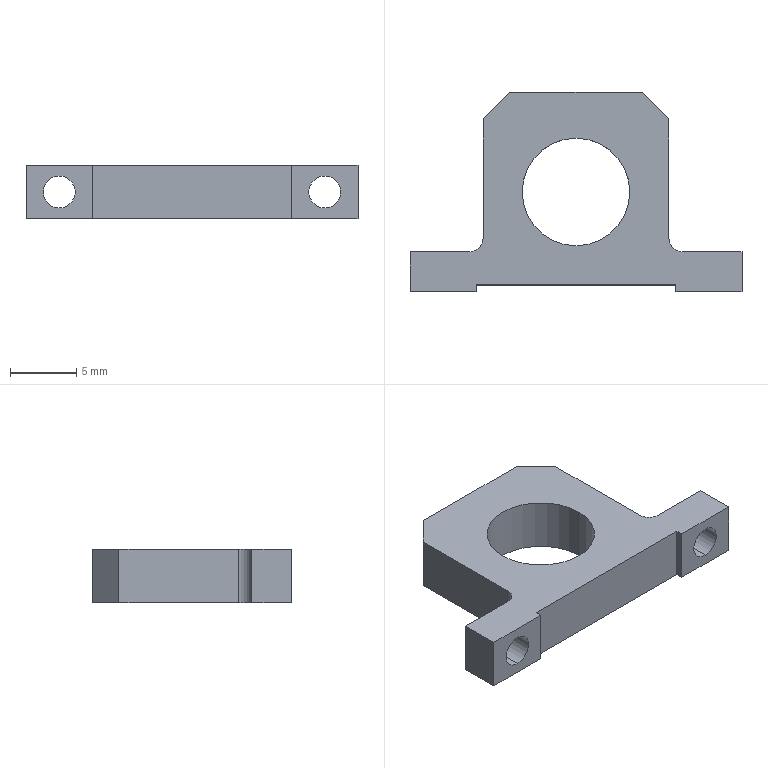Part | SolidWorks | features ICE 3, MoveFace 2, Chamfer 1, Cut 1, Extrusion 1, Fillet 1 | 1 solid | 24 faces | box 25 x 15 x 4 mm | volume 694.454 mm3 | plane 16 | cylinder 8 | commonest cylinder face diameters 2.4 x4 2 x2 8.1 x2
STEP:
#1=CARTESIAN_POINT('',(-10.,-7.5,0.8));
#2=VERTEX_POINT('',#1);
#3=CARTESIAN_POINT('',(-10.,-7.5,3.2));
#4=VERTEX_POINT('',#3);
#5=CARTESIAN_POINT('',(-10.,-7.5,2.));
#6=DIRECTION('',(0.,1.,0.));
#7=DIRECTION('',(0.,0.,1.));
#8=AXIS2_PLACEMENT_3D('',#5,#6,#7);
#9=CIRCLE('',#8,1.2);
#10=EDGE_CURVE('',#2,#4,#9,.T.);
#11=ORIENTED_EDGE('',*,*,#10,.F.);
#12=CARTESIAN_POINT('',(-10.,-4.5,0.8));
#13=VERTEX_POINT('',#12);
#14=CARTESIAN_POINT('',(-10.,-14.5,0.8));
#15=DIRECTION('',(0.,1.,0.));
#16=VECTOR('',#15,1000.);
#17=LINE('',#14,#16);
#18=EDGE_CURVE('',#2,#13,#17,.T.);
#19=ORIENTED_EDGE('',*,*,#18,.T.);
#20=CARTESIAN_POINT('',(-10.,-4.5,3.2));
#21=VERTEX_POINT('',#20);
#22=CARTESIAN_POINT('',(-10.,-4.5,2.));
#23=DIRECTION('',(0.,1.,0.));
#24=DIRECTION('',(0.,0.,1.));
#25=AXIS2_PLACEMENT_3D('',#22,#23,#24);
#26=CIRCLE('',#25,1.2);
#27=EDGE_CURVE('',#13,#21,#26,.T.);
#28=ORIENTED_EDGE('',*,*,#27,.T.);
#29=CARTESIAN_POINT('',(-10.,-14.5,3.2));
#30=DIRECTION('',(0.,1.,0.));
#31=VECTOR('',#30,1000.);
#32=LINE('',#29,#31);
#33=EDGE_CURVE('',#4,#21,#32,.T.);
#34=ORIENTED_EDGE('',*,*,#33,.F.);
#35=EDGE_LOOP('',(#11,#19,#28,#34));
#36=FACE_OUTER_BOUND('',#35,.T.);
#37=CARTESIAN_POINT('',(-10.,-14.5,2.));
#38=DIRECTION('',(0.,1.,0.));
#39=DIRECTION('',(0.,0.,1.));
#40=AXIS2_PLACEMENT_3D('',#37,#38,#39);
#41=CYLINDRICAL_SURFACE('',#40,1.2);
#42=ADVANCED_FACE('',(#36),#41,.F.);
#43=CARTESIAN_POINT('',(10.,-7.5,0.8));
#44=VERTEX_POINT('',#43);
#45=CARTESIAN_POINT('',(10.,-7.5,3.2));
#46=VERTEX_POINT('',#45);
#47=CARTESIAN_POINT('',(10.,-7.5,2.));
#48=DIRECTION('',(0.,1.,0.));
#49=DIRECTION('',(0.,0.,1.));
#50=AXIS2_PLACEMENT_3D('',#47,#48,#49);
#51=CIRCLE('',#50,1.2);
#52=EDGE_CURVE('',#44,#46,#51,.T.);
#53=ORIENTED_EDGE('',*,*,#52,.F.);
#54=CARTESIAN_POINT('',(10.,-4.5,0.8));
#55=VERTEX_POINT('',#54);
#56=CARTESIAN_POINT('',(10.,-14.5,0.8));
#57=DIRECTION('',(0.,1.,0.));
#58=VECTOR('',#57,1000.);
#59=LINE('',#56,#58);
#60=EDGE_CURVE('',#44,#55,#59,.T.);
#61=ORIENTED_EDGE('',*,*,#60,.T.);
#62=CARTESIAN_POINT('',(10.,-4.5,3.2));
#63=VERTEX_POINT('',#62);
#64=CARTESIAN_POINT('',(10.,-4.5,2.));
#65=DIRECTION('',(0.,1.,0.));
#66=DIRECTION('',(0.,0.,1.));
#67=AXIS2_PLACEMENT_3D('',#64,#65,#66);
#68=CIRCLE('',#67,1.2);
#69=EDGE_CURVE('',#55,#63,#68,.T.);
#70=ORIENTED_EDGE('',*,*,#69,.T.);
#71=CARTESIAN_POINT('',(10.,-14.5,3.2));
#72=DIRECTION('',(0.,1.,0.));
#73=VECTOR('',#72,1000.);
#74=LINE('',#71,#73);
#75=EDGE_CURVE('',#46,#63,#74,.T.);
#76=ORIENTED_EDGE('',*,*,#75,.F.);
#77=EDGE_LOOP('',(#53,#61,#70,#76));
#78=FACE_OUTER_BOUND('',#77,.T.);
#79=CARTESIAN_POINT('',(10.,-14.5,2.));
#80=DIRECTION('',(0.,1.,0.));
#81=DIRECTION('',(0.,0.,1.));
#82=AXIS2_PLACEMENT_3D('',#79,#80,#81);
#83=CYLINDRICAL_SURFACE('',#82,1.2);
#84=ADVANCED_FACE('',(#78),#83,.F.);
#85=CARTESIAN_POINT('',(-4.05,0.,0.));
#86=VERTEX_POINT('',#85);
#87=CARTESIAN_POINT('',(4.05,0.,0.));
#88=VERTEX_POINT('',#87);
#89=CARTESIAN_POINT('',(0.,0.,0.));
#90=DIRECTION('',(0.,0.,1.));
#91=DIRECTION('',(1.,0.,0.));
#92=AXIS2_PLACEMENT_3D('',#89,#90,#91);
#93=CIRCLE('',#92,4.05);
#94=EDGE_CURVE('',#86,#88,#93,.T.);
#95=ORIENTED_EDGE('',*,*,#94,.F.);
#96=CARTESIAN_POINT('',(-4.05,0.,4.));
#97=VERTEX_POINT('',#96);
#98=CARTESIAN_POINT('',(-4.05,0.,0.));
#99=DIRECTION('',(0.,0.,1.));
#100=VECTOR('',#99,1000.);
#101=LINE('',#98,#100);
#102=EDGE_CURVE('',#86,#97,#101,.T.);
#103=ORIENTED_EDGE('',*,*,#102,.T.);
#104=CARTESIAN_POINT('',(4.05,0.,4.));
#105=VERTEX_POINT('',#104);
#106=CARTESIAN_POINT('',(0.,0.,4.));
#107=DIRECTION('',(0.,0.,1.));
#108=DIRECTION('',(1.,0.,0.));
#109=AXIS2_PLACEMENT_3D('',#106,#107,#108);
#110=CIRCLE('',#109,4.05);
#111=EDGE_CURVE('',#97,#105,#110,.T.);
#112=ORIENTED_EDGE('',*,*,#111,.T.);
#113=CARTESIAN_POINT('',(4.05,0.,0.));
#114=DIRECTION('',(0.,0.,1.));
#115=VECTOR('',#114,1000.);
#116=LINE('',#113,#115);
#117=EDGE_CURVE('',#88,#105,#116,.T.);
#118=ORIENTED_EDGE('',*,*,#117,.F.);
#119=EDGE_LOOP('',(#95,#103,#112,#118));
#120=FACE_OUTER_BOUND('',#119,.T.);
#121=CARTESIAN_POINT('',(0.,0.,0.));
#122=DIRECTION('',(0.,0.,1.));
#123=DIRECTION('',(1.,0.,0.));
#124=AXIS2_PLACEMENT_3D('',#121,#122,#123);
#125=CYLINDRICAL_SURFACE('',#124,4.05);
#126=ADVANCED_FACE('',(#120),#125,.F.);
#127=CARTESIAN_POINT('',(-10.,-7.5,2.));
#128=DIRECTION('',(0.,1.,0.));
#129=DIRECTION('',(0.,0.,1.));
#130=AXIS2_PLACEMENT_3D('',#127,#128,#129);
#131=CIRCLE('',#130,1.2);
#132=EDGE_CURVE('',#4,#2,#131,.T.);
#133=ORIENTED_EDGE('',*,*,#132,.T.);
#134=ORIENTED_EDGE('',*,*,#10,.T.);
#135=EDGE_LOOP('',(#133,#134));
#136=FACE_BOUND('',#135,.T.);
#137=CARTESIAN_POINT('',(-12.5,-7.5,0.));
#138=VERTEX_POINT('',#137);
#139=CARTESIAN_POINT('',(-7.5,-7.5,0.));
#140=VERTEX_POINT('',#139);
#141=CARTESIAN_POINT('',(-7.5,-7.5,0.));
#142=DIRECTION('',(1.,0.,0.));
#143=VECTOR('',#142,1000.);
#144=LINE('',#141,#143);
#145=EDGE_CURVE('',#138,#140,#144,.T.);
#146=ORIENTED_EDGE('',*,*,#145,.T.);
#147=CARTESIAN_POINT('',(-7.5,-7.5,4.));
#148=VERTEX_POINT('',#147);
#149=CARTESIAN_POINT('',(-7.5,-7.5,-6.));
#150=DIRECTION('',(0.,0.,1.));
#151=VECTOR('',#150,1000.);
#152=LINE('',#149,#151);
#153=EDGE_CURVE('',#140,#148,#152,.T.);
#154=ORIENTED_EDGE('',*,*,#153,.T.);
#155=CARTESIAN_POINT('',(-12.5,-7.5,4.));
#156=VERTEX_POINT('',#155);
#157=CARTESIAN_POINT('',(-7.5,-7.5,4.));
#158=DIRECTION('',(1.,0.,0.));
#159=VECTOR('',#158,1000.);
#160=LINE('',#157,#159);
#161=EDGE_CURVE('',#156,#148,#160,.T.);
#162=ORIENTED_EDGE('',*,*,#161,.F.);
#163=CARTESIAN_POINT('',(-12.5,-7.5,0.));
#164=DIRECTION('',(0.,0.,-1.));
#165=VECTOR('',#164,1000.);
#166=LINE('',#163,#165);
#167=EDGE_CURVE('',#156,#138,#166,.T.);
#168=ORIENTED_EDGE('',*,*,#167,.T.);
#169=EDGE_LOOP('',(#146,#154,#162,#168));
#170=FACE_OUTER_BOUND('',#169,.T.);
#171=CARTESIAN_POINT('',(-7.5,-7.5,4.));
#172=DIRECTION('',(0.,1.,0.));
#173=DIRECTION('',(0.,0.,1.));
#174=AXIS2_PLACEMENT_3D('',#171,#172,#173);
#175=PLANE('',#174);
#176=ADVANCED_FACE('',(#136,#170),#175,.F.);
#177=CARTESIAN_POINT('',(7.,-3.5,4.));
#178=VERTEX_POINT('',#177);
#179=CARTESIAN_POINT('',(7.,5.5,4.));
#180=VERTEX_POINT('',#179);
#181=CARTESIAN_POINT('',(7.,7.5,4.));
#182=DIRECTION('',(0.,1.,0.));
#183=VECTOR('',#182,1000.);
#184=LINE('',#181,#183);
#185=EDGE_CURVE('',#178,#180,#184,.T.);
#186=ORIENTED_EDGE('',*,*,#185,.F.);
#187=CARTESIAN_POINT('',(7.,-3.5,0.));
#188=VERTEX_POINT('',#187);
#189=CARTESIAN_POINT('',(7.,-3.5,4.));
#190=DIRECTION('',(0.,0.,-1.));
#191=VECTOR('',#190,1000.);
#192=LINE('',#189,#191);
#193=EDGE_CURVE('',#178,#188,#192,.T.);
#194=ORIENTED_EDGE('',*,*,#193,.T.);
#195=CARTESIAN_POINT('',(7.,5.5,0.));
#196=VERTEX_POINT('',#195);
#197=CARTESIAN_POINT('',(7.,7.5,0.));
#198=DIRECTION('',(0.,1.,0.));
#199=VECTOR('',#198,1000.);
#200=LINE('',#197,#199);
#201=EDGE_CURVE('',#188,#196,#200,.T.);
#202=ORIENTED_EDGE('',*,*,#201,.T.);
#203=CARTESIAN_POINT('',(7.,5.5,4.));
#204=DIRECTION('',(0.,0.,1.));
#205=VECTOR('',#204,1000.);
#206=LINE('',#203,#205);
#207=EDGE_CURVE('',#196,#180,#206,.T.);
#208=ORIENTED_EDGE('',*,*,#207,.T.);
#209=EDGE_LOOP('',(#186,#194,#202,#208));
#210=FACE_OUTER_BOUND('',#209,.T.);
#211=CARTESIAN_POINT('',(7.,7.5,4.));
#212=DIRECTION('',(-1.,0.,0.));
#213=DIRECTION('',(0.,0.,1.));
#214=AXIS2_PLACEMENT_3D('',#211,#212,#213);
#215=PLANE('',#214);
#216=ADVANCED_FACE('',(#210),#215,.F.);
#217=CARTESIAN_POINT('',(5.,7.5,4.));
#218=VERTEX_POINT('',#217);
#219=CARTESIAN_POINT('',(-5.,7.5,4.));
#220=VERTEX_POINT('',#219);
#221=CARTESIAN_POINT('',(-7.5,7.5,4.));
#222=DIRECTION('',(-1.,0.,0.));
#223=VECTOR('',#222,1000.);
#224=LINE('',#221,#223);
#225=EDGE_CURVE('',#218,#220,#224,.T.);
#226=ORIENTED_EDGE('',*,*,#225,.F.);
#227=CARTESIAN_POINT('',(5.,7.5,0.));
#228=VERTEX_POINT('',#227);
#229=CARTESIAN_POINT('',(5.,7.5,4.));
#230=DIRECTION('',(0.,0.,-1.));
#231=VECTOR('',#230,1000.);
#232=LINE('',#229,#231);
#233=EDGE_CURVE('',#218,#228,#232,.T.);
#234=ORIENTED_EDGE('',*,*,#233,.T.);
#235=CARTESIAN_POINT('',(-5.,7.5,0.));
#236=VERTEX_POINT('',#235);
#237=CARTESIAN_POINT('',(-7.5,7.5,0.));
#238=DIRECTION('',(-1.,0.,0.));
#239=VECTOR('',#238,1000.);
#240=LINE('',#237,#239);
#241=EDGE_CURVE('',#228,#236,#240,.T.);
#242=ORIENTED_EDGE('',*,*,#241,.T.);
#243=CARTESIAN_POINT('',(-5.,7.5,4.));
#244=DIRECTION('',(0.,0.,1.));
#245=VECTOR('',#244,1000.);
#246=LINE('',#243,#245);
#247=EDGE_CURVE('',#236,#220,#246,.T.);
#248=ORIENTED_EDGE('',*,*,#247,.T.);
#249=EDGE_LOOP('',(#226,#234,#242,#248));
#250=FACE_OUTER_BOUND('',#249,.T.);
#251=CARTESIAN_POINT('',(-7.5,7.5,4.));
#252=DIRECTION('',(0.,-1.,0.));
#253=DIRECTION('',(0.,0.,-1.));
#254=AXIS2_PLACEMENT_3D('',#251,#252,#253);
#255=PLANE('',#254);
#256=ADVANCED_FACE('',(#250),#255,.F.);
#257=CARTESIAN_POINT('',(-7.,5.5,0.));
#258=VERTEX_POINT('',#257);
#259=CARTESIAN_POINT('',(-7.,-3.5,0.));
#260=VERTEX_POINT('',#259);
#261=CARTESIAN_POINT('',(-7.,7.5,0.));
#262=DIRECTION('',(0.,-1.,0.));
#263=VECTOR('',#262,1000.);
#264=LINE('',#261,#263);
#265=EDGE_CURVE('',#258,#260,#264,.T.);
#266=ORIENTED_EDGE('',*,*,#265,.T.);
#267=CARTESIAN_POINT('',(-7.,-3.5,4.));
#268=VERTEX_POINT('',#267);
#269=CARTESIAN_POINT('',(-7.,-3.5,4.));
#270=DIRECTION('',(0.,0.,1.));
#271=VECTOR('',#270,1000.);
#272=LINE('',#269,#271);
#273=EDGE_CURVE('',#260,#268,#272,.T.);
#274=ORIENTED_EDGE('',*,*,#273,.T.);
#275=CARTESIAN_POINT('',(-7.,5.5,4.));
#276=VERTEX_POINT('',#275);
#277=CARTESIAN_POINT('',(-7.,7.5,4.));
#278=DIRECTION('',(0.,-1.,0.));
#279=VECTOR('',#278,1000.);
#280=LINE('',#277,#279);
#281=EDGE_CURVE('',#276,#268,#280,.T.);
#282=ORIENTED_EDGE('',*,*,#281,.F.);
#283=CARTESIAN_POINT('',(-7.,5.5,4.));
#284=DIRECTION('',(0.,0.,-1.));
#285=VECTOR('',#284,1000.);
#286=LINE('',#283,#285);
#287=EDGE_CURVE('',#276,#258,#286,.T.);
#288=ORIENTED_EDGE('',*,*,#287,.T.);
#289=EDGE_LOOP('',(#266,#274,#282,#288));
#290=FACE_OUTER_BOUND('',#289,.T.);
#291=CARTESIAN_POINT('',(-7.,7.5,4.));
#292=DIRECTION('',(1.,0.,0.));
#293=DIRECTION('',(0.,1.,0.));
#294=AXIS2_PLACEMENT_3D('',#291,#292,#293);
#295=PLANE('',#294);
#296=ADVANCED_FACE('',(#290),#295,.F.);
#297=CARTESIAN_POINT('',(10.,-7.5,2.));
#298=DIRECTION('',(0.,1.,0.));
#299=DIRECTION('',(0.,0.,1.));
#300=AXIS2_PLACEMENT_3D('',#297,#298,#299);
#301=CIRCLE('',#300,1.2);
#302=EDGE_CURVE('',#46,#44,#301,.T.);
#303=ORIENTED_EDGE('',*,*,#302,.T.);
#304=ORIENTED_EDGE('',*,*,#52,.T.);
#305=EDGE_LOOP('',(#303,#304));
#306=FACE_BOUND('',#305,.T.);
#307=CARTESIAN_POINT('',(7.5,-7.5,4.));
#308=VERTEX_POINT('',#307);
#309=CARTESIAN_POINT('',(12.5,-7.5,4.));
#310=VERTEX_POINT('',#309);
#311=CARTESIAN_POINT('',(-7.5,-7.5,4.));
#312=DIRECTION('',(1.,0.,0.));
#313=VECTOR('',#312,1000.);
#314=LINE('',#311,#313);
#315=EDGE_CURVE('',#308,#310,#314,.T.);
#316=ORIENTED_EDGE('',*,*,#315,.F.);
#317=CARTESIAN_POINT('',(7.5,-7.5,0.));
#318=VERTEX_POINT('',#317);
#319=CARTESIAN_POINT('',(7.5,-7.5,-6.));
#320=DIRECTION('',(0.,0.,1.));
#321=VECTOR('',#320,1000.);
#322=LINE('',#319,#321);
#323=EDGE_CURVE('',#318,#308,#322,.T.);
#324=ORIENTED_EDGE('',*,*,#323,.F.);
#325=CARTESIAN_POINT('',(12.5,-7.5,0.));
#326=VERTEX_POINT('',#325);
#327=CARTESIAN_POINT('',(-7.5,-7.5,0.));
#328=DIRECTION('',(1.,0.,0.));
#329=VECTOR('',#328,1000.);
#330=LINE('',#327,#329);
#331=EDGE_CURVE('',#318,#326,#330,.T.);
#332=ORIENTED_EDGE('',*,*,#331,.T.);
#333=CARTESIAN_POINT('',(12.5,-7.5,4.));
#334=DIRECTION('',(0.,0.,1.));
#335=VECTOR('',#334,1000.);
#336=LINE('',#333,#335);
#337=EDGE_CURVE('',#326,#310,#336,.T.);
#338=ORIENTED_EDGE('',*,*,#337,.T.);
#339=EDGE_LOOP('',(#316,#324,#332,#338));
#340=FACE_OUTER_BOUND('',#339,.T.);
#341=CARTESIAN_POINT('',(-7.5,-7.5,4.));
#342=DIRECTION('',(0.,1.,0.));
#343=DIRECTION('',(0.,0.,1.));
#344=AXIS2_PLACEMENT_3D('',#341,#342,#343);
#345=PLANE('',#344);
#346=ADVANCED_FACE('',(#306,#340),#345,.F.);
#347=CARTESIAN_POINT('',(-7.5,-7.,4.));
#348=VERTEX_POINT('',#347);
#349=CARTESIAN_POINT('',(-7.5,-7.5,4.));
#350=DIRECTION('',(0.,-1.,0.));
#351=VECTOR('',#350,1000.);
#352=LINE('',#349,#351);
#353=EDGE_CURVE('',#348,#148,#352,.T.);
#354=ORIENTED_EDGE('',*,*,#353,.F.);
#355=CARTESIAN_POINT('',(7.5,-7.,4.));
#356=VERTEX_POINT('',#355);
#357=CARTESIAN_POINT('',(-7.5,-7.,4.));
#358=DIRECTION('',(-1.,0.,0.));
#359=VECTOR('',#358,1000.);
#360=LINE('',#357,#359);
#361=EDGE_CURVE('',#356,#348,#360,.T.);
#362=ORIENTED_EDGE('',*,*,#361,.F.);
#363=CARTESIAN_POINT('',(7.5,-7.,4.));
#364=DIRECTION('',(0.,1.,0.));
#365=VECTOR('',#364,1000.);
#366=LINE('',#363,#365);
#367=EDGE_CURVE('',#308,#356,#366,.T.);
#368=ORIENTED_EDGE('',*,*,#367,.F.);
#369=ORIENTED_EDGE('',*,*,#315,.T.);
#370=CARTESIAN_POINT('',(12.5,-4.5,4.));
#371=VERTEX_POINT('',#370);
#372=CARTESIAN_POINT('',(12.5,-4.5,4.));
#373=DIRECTION('',(0.,-1.,0.));
#374=VECTOR('',#373,1000.);
#375=LINE('',#372,#374);
#376=EDGE_CURVE('',#371,#310,#375,.T.);
#377=ORIENTED_EDGE('',*,*,#376,.F.);
#378=CARTESIAN_POINT('',(8.,-4.5,4.));
#379=VERTEX_POINT('',#378);
#380=CARTESIAN_POINT('',(7.5,-4.5,4.));
#381=DIRECTION('',(-1.,0.,0.));
#382=VECTOR('',#381,1000.);
#383=LINE('',#380,#382);
#384=EDGE_CURVE('',#371,#379,#383,.T.);
#385=ORIENTED_EDGE('',*,*,#384,.T.);
#386=CARTESIAN_POINT('',(8.,-3.5,4.));
#387=DIRECTION('',(0.,0.,-1.));
#388=DIRECTION('',(1.,0.,0.));
#389=AXIS2_PLACEMENT_3D('',#386,#387,#388);
#390=CIRCLE('',#389,1.);
#391=EDGE_CURVE('',#379,#178,#390,.T.);
#392=ORIENTED_EDGE('',*,*,#391,.T.);
#393=ORIENTED_EDGE('',*,*,#185,.T.);
#394=CARTESIAN_POINT('',(6.,6.5,4.));
#395=DIRECTION('',(-0.7071,0.7071,0.));
#396=VECTOR('',#395,1000.);
#397=LINE('',#394,#396);
#398=EDGE_CURVE('',#180,#218,#397,.T.);
#399=ORIENTED_EDGE('',*,*,#398,.T.);
#400=ORIENTED_EDGE('',*,*,#225,.T.);
#401=CARTESIAN_POINT('',(-6.,6.5,4.));
#402=DIRECTION('',(-0.7071,-0.7071,0.));
#403=VECTOR('',#402,1000.);
#404=LINE('',#401,#403);
#405=EDGE_CURVE('',#220,#276,#404,.T.);
#406=ORIENTED_EDGE('',*,*,#405,.T.);
#407=ORIENTED_EDGE('',*,*,#281,.T.);
#408=CARTESIAN_POINT('',(-8.,-4.5,4.));
#409=VERTEX_POINT('',#408);
#410=CARTESIAN_POINT('',(-8.,-3.5,4.));
#411=DIRECTION('',(0.,0.,-1.));
#412=DIRECTION('',(1.,0.,0.));
#413=AXIS2_PLACEMENT_3D('',#410,#411,#412);
#414=CIRCLE('',#413,1.);
#415=EDGE_CURVE('',#268,#409,#414,.T.);
#416=ORIENTED_EDGE('',*,*,#415,.T.);
#417=CARTESIAN_POINT('',(-12.5,-4.5,4.));
#418=VERTEX_POINT('',#417);
#419=CARTESIAN_POINT('',(-12.5,-4.5,4.));
#420=DIRECTION('',(-1.,0.,0.));
#421=VECTOR('',#420,1000.);
#422=LINE('',#419,#421);
#423=EDGE_CURVE('',#409,#418,#422,.T.);
#424=ORIENTED_EDGE('',*,*,#423,.T.);
#425=CARTESIAN_POINT('',(-12.5,-4.5,4.));
#426=DIRECTION('',(0.,-1.,0.));
#427=VECTOR('',#426,1000.);
#428=LINE('',#425,#427);
#429=EDGE_CURVE('',#418,#156,#428,.T.);
#430=ORIENTED_EDGE('',*,*,#429,.T.);
#431=ORIENTED_EDGE('',*,*,#161,.T.);
#432=EDGE_LOOP('',(#354,#362,#368,#369,#377,#385,#392,#393,#399,#400,#406,#407,#416,#424,#430,#431));
#433=FACE_OUTER_BOUND('',#432,.T.);
#434=CARTESIAN_POINT('',(0.,0.,4.));
#435=DIRECTION('',(0.,0.,1.));
#436=DIRECTION('',(1.,0.,0.));
#437=AXIS2_PLACEMENT_3D('',#434,#435,#436);
#438=CIRCLE('',#437,4.05);
#439=EDGE_CURVE('',#105,#97,#438,.T.);
#440=ORIENTED_EDGE('',*,*,#439,.F.);
#441=ORIENTED_EDGE('',*,*,#111,.F.);
#442=EDGE_LOOP('',(#440,#441));
#443=FACE_BOUND('',#442,.T.);
#444=CARTESIAN_POINT('',(0.,0.,4.));
#445=DIRECTION('',(0.,0.,1.));
#446=DIRECTION('',(1.,0.,0.));
#447=AXIS2_PLACEMENT_3D('',#444,#445,#446);
#448=PLANE('',#447);
#449=ADVANCED_FACE('',(#433,#443),#448,.T.);
#450=CARTESIAN_POINT('',(0.,0.,0.));
#451=DIRECTION('',(0.,0.,1.));
#452=DIRECTION('',(1.,0.,0.));
#453=AXIS2_PLACEMENT_3D('',#450,#451,#452);
#454=CIRCLE('',#453,4.05);
#455=EDGE_CURVE('',#88,#86,#454,.T.);
#456=ORIENTED_EDGE('',*,*,#455,.T.);
#457=ORIENTED_EDGE('',*,*,#94,.T.);
#458=EDGE_LOOP('',(#456,#457));
#459=FACE_BOUND('',#458,.T.);
#460=CARTESIAN_POINT('',(7.5,-7.,0.));
#461=VERTEX_POINT('',#460);
#462=CARTESIAN_POINT('',(-7.5,-7.,0.));
#463=VERTEX_POINT('',#462);
#464=CARTESIAN_POINT('',(0.,-7.,0.));
#465=DIRECTION('',(-1.,0.,0.));
#466=VECTOR('',#465,1000.);
#467=LINE('',#464,#466);
#468=EDGE_CURVE('',#461,#463,#467,.T.);
#469=ORIENTED_EDGE('',*,*,#468,.T.);
#470=CARTESIAN_POINT('',(-7.5,0.,0.));
#471=DIRECTION('',(0.,-1.,0.));
#472=VECTOR('',#471,1000.);
#473=LINE('',#470,#472);
#474=EDGE_CURVE('',#463,#140,#473,.T.);
#475=ORIENTED_EDGE('',*,*,#474,.T.);
#476=ORIENTED_EDGE('',*,*,#145,.F.);
#477=CARTESIAN_POINT('',(-12.5,-4.5,0.));
#478=VERTEX_POINT('',#477);
#479=CARTESIAN_POINT('',(-12.5,-4.5,0.));
#480=DIRECTION('',(0.,-1.,0.));
#481=VECTOR('',#480,1000.);
#482=LINE('',#479,#481);
#483=EDGE_CURVE('',#478,#138,#482,.T.);
#484=ORIENTED_EDGE('',*,*,#483,.F.);
#485=CARTESIAN_POINT('',(-8.,-4.5,0.));
#486=VERTEX_POINT('',#485);
#487=CARTESIAN_POINT('',(-7.5,-4.5,0.));
#488=DIRECTION('',(1.,0.,0.));
#489=VECTOR('',#488,1000.);
#490=LINE('',#487,#489);
#491=EDGE_CURVE('',#478,#486,#490,.T.);
#492=ORIENTED_EDGE('',*,*,#491,.T.);
#493=CARTESIAN_POINT('',(-8.,-3.5,0.));
#494=DIRECTION('',(0.,0.,1.));
#495=DIRECTION('',(1.,0.,0.));
#496=AXIS2_PLACEMENT_3D('',#493,#494,#495);
#497=CIRCLE('',#496,1.);
#498=EDGE_CURVE('',#486,#260,#497,.T.);
#499=ORIENTED_EDGE('',*,*,#498,.T.);
#500=ORIENTED_EDGE('',*,*,#265,.F.);
#501=CARTESIAN_POINT('',(-7.,5.5,0.));
#502=DIRECTION('',(0.7071,0.7071,0.));
#503=VECTOR('',#502,1000.);
#504=LINE('',#501,#503);
#505=EDGE_CURVE('',#258,#236,#504,.T.);
#506=ORIENTED_EDGE('',*,*,#505,.T.);
#507=ORIENTED_EDGE('',*,*,#241,.F.);
#508=CARTESIAN_POINT('',(5.,7.5,0.));
#509=DIRECTION('',(0.7071,-0.7071,0.));
#510=VECTOR('',#509,1000.);
#511=LINE('',#508,#510);
#512=EDGE_CURVE('',#228,#196,#511,.T.);
#513=ORIENTED_EDGE('',*,*,#512,.T.);
#514=ORIENTED_EDGE('',*,*,#201,.F.);
#515=CARTESIAN_POINT('',(8.,-4.5,0.));
#516=VERTEX_POINT('',#515);
#517=CARTESIAN_POINT('',(8.,-3.5,0.));
#518=DIRECTION('',(0.,0.,1.));
#519=DIRECTION('',(1.,0.,0.));
#520=AXIS2_PLACEMENT_3D('',#517,#518,#519);
#521=CIRCLE('',#520,1.);
#522=EDGE_CURVE('',#188,#516,#521,.T.);
#523=ORIENTED_EDGE('',*,*,#522,.T.);
#524=CARTESIAN_POINT('',(12.5,-4.5,0.));
#525=VERTEX_POINT('',#524);
#526=CARTESIAN_POINT('',(12.5,-4.5,0.));
#527=DIRECTION('',(1.,0.,0.));
#528=VECTOR('',#527,1000.);
#529=LINE('',#526,#528);
#530=EDGE_CURVE('',#516,#525,#529,.T.);
#531=ORIENTED_EDGE('',*,*,#530,.T.);
#532=CARTESIAN_POINT('',(12.5,-4.5,0.));
#533=DIRECTION('',(0.,-1.,0.));
#534=VECTOR('',#533,1000.);
#535=LINE('',#532,#534);
#536=EDGE_CURVE('',#525,#326,#535,.T.);
#537=ORIENTED_EDGE('',*,*,#536,.T.);
#538=ORIENTED_EDGE('',*,*,#331,.F.);
#539=CARTESIAN_POINT('',(7.5,0.,0.));
#540=DIRECTION('',(0.,1.,0.));
#541=VECTOR('',#540,1000.);
#542=LINE('',#539,#541);
#543=EDGE_CURVE('',#318,#461,#542,.T.);
#544=ORIENTED_EDGE('',*,*,#543,.T.);
#545=EDGE_LOOP('',(#469,#475,#476,#484,#492,#499,#500,#506,#507,#513,#514,#523,#531,#537,#538,#544));
#546=FACE_OUTER_BOUND('',#545,.T.);
#547=CARTESIAN_POINT('',(0.,0.,0.));
#548=DIRECTION('',(0.,0.,1.));
#549=DIRECTION('',(1.,0.,0.));
#550=AXIS2_PLACEMENT_3D('',#547,#548,#549);
#551=PLANE('',#550);
#552=ADVANCED_FACE('',(#459,#546),#551,.F.);
#553=ORIENTED_EDGE('',*,*,#102,.F.);
#554=ORIENTED_EDGE('',*,*,#455,.F.);
#555=ORIENTED_EDGE('',*,*,#117,.T.);
#556=ORIENTED_EDGE('',*,*,#439,.T.);
#557=EDGE_LOOP('',(#553,#554,#555,#556));
#558=FACE_OUTER_BOUND('',#557,.T.);
#559=CARTESIAN_POINT('',(0.,0.,0.));
#560=DIRECTION('',(0.,0.,1.));
#561=DIRECTION('',(1.,0.,0.));
#562=AXIS2_PLACEMENT_3D('',#559,#560,#561);
#563=CYLINDRICAL_SURFACE('',#562,4.05);
#564=ADVANCED_FACE('',(#558),#563,.F.);
#565=ORIENTED_EDGE('',*,*,#398,.F.);
#566=ORIENTED_EDGE('',*,*,#207,.F.);
#567=ORIENTED_EDGE('',*,*,#512,.F.);
#568=ORIENTED_EDGE('',*,*,#233,.F.);
#569=EDGE_LOOP('',(#565,#566,#567,#568));
#570=FACE_OUTER_BOUND('',#569,.T.);
#571=CARTESIAN_POINT('',(5.,7.5,4.));
#572=DIRECTION('',(-0.7071,-0.7071,0.));
#573=DIRECTION('',(0.,0.,-1.));
#574=AXIS2_PLACEMENT_3D('',#571,#572,#573);
#575=PLANE('',#574);
#576=ADVANCED_FACE('',(#570),#575,.F.);
#577=ORIENTED_EDGE('',*,*,#405,.F.);
#578=ORIENTED_EDGE('',*,*,#247,.F.);
#579=ORIENTED_EDGE('',*,*,#505,.F.);
#580=ORIENTED_EDGE('',*,*,#287,.F.);
#581=EDGE_LOOP('',(#577,#578,#579,#580));
#582=FACE_OUTER_BOUND('',#581,.T.);
#583=CARTESIAN_POINT('',(-7.,5.5,4.));
#584=DIRECTION('',(0.7071,-0.7071,0.));
#585=DIRECTION('',(0.,0.,-1.));
#586=AXIS2_PLACEMENT_3D('',#583,#584,#585);
#587=PLANE('',#586);
#588=ADVANCED_FACE('',(#582),#587,.F.);
#589=ORIENTED_EDGE('',*,*,#167,.F.);
#590=ORIENTED_EDGE('',*,*,#429,.F.);
#591=CARTESIAN_POINT('',(-12.5,-4.5,0.));
#592=DIRECTION('',(0.,0.,-1.));
#593=VECTOR('',#592,1000.);
#594=LINE('',#591,#593);
#595=EDGE_CURVE('',#418,#478,#594,.T.);
#596=ORIENTED_EDGE('',*,*,#595,.T.);
#597=ORIENTED_EDGE('',*,*,#483,.T.);
#598=EDGE_LOOP('',(#589,#590,#596,#597));
#599=FACE_OUTER_BOUND('',#598,.T.);
#600=CARTESIAN_POINT('',(-12.5,-4.5,0.));
#601=DIRECTION('',(-1.,0.,0.));
#602=DIRECTION('',(0.,0.,1.));
#603=AXIS2_PLACEMENT_3D('',#600,#601,#602);
#604=PLANE('',#603);
#605=ADVANCED_FACE('',(#599),#604,.T.);
#606=CARTESIAN_POINT('',(-10.,-4.5,2.));
#607=DIRECTION('',(0.,1.,0.));
#608=DIRECTION('',(0.,0.,1.));
#609=AXIS2_PLACEMENT_3D('',#606,#607,#608);
#610=CIRCLE('',#609,1.2);
#611=EDGE_CURVE('',#21,#13,#610,.T.);
#612=ORIENTED_EDGE('',*,*,#611,.F.);
#613=ORIENTED_EDGE('',*,*,#27,.F.);
#614=EDGE_LOOP('',(#612,#613));
#615=FACE_BOUND('',#614,.T.);
#616=ORIENTED_EDGE('',*,*,#423,.F.);
#617=CARTESIAN_POINT('',(-8.,-4.5,0.));
#618=DIRECTION('',(0.,0.,-1.));
#619=VECTOR('',#618,1000.);
#620=LINE('',#617,#619);
#621=EDGE_CURVE('',#409,#486,#620,.T.);
#622=ORIENTED_EDGE('',*,*,#621,.T.);
#623=ORIENTED_EDGE('',*,*,#491,.F.);
#624=ORIENTED_EDGE('',*,*,#595,.F.);
#625=EDGE_LOOP('',(#616,#622,#623,#624));
#626=FACE_OUTER_BOUND('',#625,.T.);
#627=CARTESIAN_POINT('',(0.,-4.5,0.));
#628=DIRECTION('',(0.,1.,0.));
#629=DIRECTION('',(0.,0.,1.));
#630=AXIS2_PLACEMENT_3D('',#627,#628,#629);
#631=PLANE('',#630);
#632=ADVANCED_FACE('',(#615,#626),#631,.T.);
#633=ORIENTED_EDGE('',*,*,#337,.F.);
#634=ORIENTED_EDGE('',*,*,#536,.F.);
#635=CARTESIAN_POINT('',(12.5,-4.5,4.));
#636=DIRECTION('',(0.,0.,1.));
#637=VECTOR('',#636,1000.);
#638=LINE('',#635,#637);
#639=EDGE_CURVE('',#525,#371,#638,.T.);
#640=ORIENTED_EDGE('',*,*,#639,.T.);
#641=ORIENTED_EDGE('',*,*,#376,.T.);
#642=EDGE_LOOP('',(#633,#634,#640,#641));
#643=FACE_OUTER_BOUND('',#642,.T.);
#644=CARTESIAN_POINT('',(12.5,-4.5,4.));
#645=DIRECTION('',(1.,0.,0.));
#646=DIRECTION('',(0.,0.,-1.));
#647=AXIS2_PLACEMENT_3D('',#644,#645,#646);
#648=PLANE('',#647);
#649=ADVANCED_FACE('',(#643),#648,.T.);
#650=CARTESIAN_POINT('',(10.,-4.5,2.));
#651=DIRECTION('',(0.,1.,0.));
#652=DIRECTION('',(0.,0.,1.));
#653=AXIS2_PLACEMENT_3D('',#650,#651,#652);
#654=CIRCLE('',#653,1.2);
#655=EDGE_CURVE('',#63,#55,#654,.T.);
#656=ORIENTED_EDGE('',*,*,#655,.F.);
#657=ORIENTED_EDGE('',*,*,#69,.F.);
#658=EDGE_LOOP('',(#656,#657));
#659=FACE_BOUND('',#658,.T.);
#660=ORIENTED_EDGE('',*,*,#530,.F.);
#661=CARTESIAN_POINT('',(8.,-4.5,0.));
#662=DIRECTION('',(0.,0.,1.));
#663=VECTOR('',#662,1000.);
#664=LINE('',#661,#663);
#665=EDGE_CURVE('',#516,#379,#664,.T.);
#666=ORIENTED_EDGE('',*,*,#665,.T.);
#667=ORIENTED_EDGE('',*,*,#384,.F.);
#668=ORIENTED_EDGE('',*,*,#639,.F.);
#669=EDGE_LOOP('',(#660,#666,#667,#668));
#670=FACE_OUTER_BOUND('',#669,.T.);
#671=CARTESIAN_POINT('',(0.,-4.5,0.));
#672=DIRECTION('',(0.,1.,0.));
#673=DIRECTION('',(0.,0.,1.));
#674=AXIS2_PLACEMENT_3D('',#671,#672,#673);
#675=PLANE('',#674);
#676=ADVANCED_FACE('',(#659,#670),#675,.T.);
#677=ORIENTED_EDGE('',*,*,#60,.F.);
#678=ORIENTED_EDGE('',*,*,#302,.F.);
#679=ORIENTED_EDGE('',*,*,#75,.T.);
#680=ORIENTED_EDGE('',*,*,#655,.T.);
#681=EDGE_LOOP('',(#677,#678,#679,#680));
#682=FACE_OUTER_BOUND('',#681,.T.);
#683=CARTESIAN_POINT('',(10.,-14.5,2.));
#684=DIRECTION('',(0.,1.,0.));
#685=DIRECTION('',(0.,0.,1.));
#686=AXIS2_PLACEMENT_3D('',#683,#684,#685);
#687=CYLINDRICAL_SURFACE('',#686,1.2);
#688=ADVANCED_FACE('',(#682),#687,.F.);
#689=ORIENTED_EDGE('',*,*,#18,.F.);
#690=ORIENTED_EDGE('',*,*,#132,.F.);
#691=ORIENTED_EDGE('',*,*,#33,.T.);
#692=ORIENTED_EDGE('',*,*,#611,.T.);
#693=EDGE_LOOP('',(#689,#690,#691,#692));
#694=FACE_OUTER_BOUND('',#693,.T.);
#695=CARTESIAN_POINT('',(-10.,-14.5,2.));
#696=DIRECTION('',(0.,1.,0.));
#697=DIRECTION('',(0.,0.,1.));
#698=AXIS2_PLACEMENT_3D('',#695,#696,#697);
#699=CYLINDRICAL_SURFACE('',#698,1.2);
#700=ADVANCED_FACE('',(#694),#699,.F.);
#701=ORIENTED_EDGE('',*,*,#391,.F.);
#702=ORIENTED_EDGE('',*,*,#665,.F.);
#703=ORIENTED_EDGE('',*,*,#522,.F.);
#704=ORIENTED_EDGE('',*,*,#193,.F.);
#705=EDGE_LOOP('',(#701,#702,#703,#704));
#706=FACE_OUTER_BOUND('',#705,.T.);
#707=CARTESIAN_POINT('',(8.,-3.5,4.));
#708=DIRECTION('',(0.,0.,-1.));
#709=DIRECTION('',(-1.,0.,0.));
#710=AXIS2_PLACEMENT_3D('',#707,#708,#709);
#711=CYLINDRICAL_SURFACE('',#710,1.);
#712=ADVANCED_FACE('',(#706),#711,.F.);
#713=ORIENTED_EDGE('',*,*,#498,.F.);
#714=ORIENTED_EDGE('',*,*,#621,.F.);
#715=ORIENTED_EDGE('',*,*,#415,.F.);
#716=ORIENTED_EDGE('',*,*,#273,.F.);
#717=EDGE_LOOP('',(#713,#714,#715,#716));
#718=FACE_OUTER_BOUND('',#717,.T.);
#719=CARTESIAN_POINT('',(-8.,-3.5,4.));
#720=DIRECTION('',(0.,0.,1.));
#721=DIRECTION('',(1.,0.,0.));
#722=AXIS2_PLACEMENT_3D('',#719,#720,#721);
#723=CYLINDRICAL_SURFACE('',#722,1.);
#724=ADVANCED_FACE('',(#718),#723,.F.);
#725=CARTESIAN_POINT('',(-7.5,-7.,-6.));
#726=DIRECTION('',(0.,0.,1.));
#727=VECTOR('',#726,1000.);
#728=LINE('',#725,#727);
#729=EDGE_CURVE('',#463,#348,#728,.T.);
#730=ORIENTED_EDGE('',*,*,#729,.T.);
#731=ORIENTED_EDGE('',*,*,#353,.T.);
#732=ORIENTED_EDGE('',*,*,#153,.F.);
#733=ORIENTED_EDGE('',*,*,#474,.F.);
#734=EDGE_LOOP('',(#730,#731,#732,#733));
#735=FACE_OUTER_BOUND('',#734,.T.);
#736=CARTESIAN_POINT('',(-7.5,-7.5,-6.));
#737=DIRECTION('',(-1.,0.,0.));
#738=DIRECTION('',(0.,0.,1.));
#739=AXIS2_PLACEMENT_3D('',#736,#737,#738);
#740=PLANE('',#739);
#741=ADVANCED_FACE('',(#735),#740,.F.);
#742=CARTESIAN_POINT('',(7.5,-7.,-6.));
#743=DIRECTION('',(0.,0.,1.));
#744=VECTOR('',#743,1000.);
#745=LINE('',#742,#744);
#746=EDGE_CURVE('',#461,#356,#745,.T.);
#747=ORIENTED_EDGE('',*,*,#746,.T.);
#748=ORIENTED_EDGE('',*,*,#361,.T.);
#749=ORIENTED_EDGE('',*,*,#729,.F.);
#750=ORIENTED_EDGE('',*,*,#468,.F.);
#751=EDGE_LOOP('',(#747,#748,#749,#750));
#752=FACE_OUTER_BOUND('',#751,.T.);
#753=CARTESIAN_POINT('',(-7.5,-7.,-6.));
#754=DIRECTION('',(0.,1.,0.));
#755=DIRECTION('',(0.,0.,1.));
#756=AXIS2_PLACEMENT_3D('',#753,#754,#755);
#757=PLANE('',#756);
#758=ADVANCED_FACE('',(#752),#757,.F.);
#759=ORIENTED_EDGE('',*,*,#323,.T.);
#760=ORIENTED_EDGE('',*,*,#367,.T.);
#761=ORIENTED_EDGE('',*,*,#746,.F.);
#762=ORIENTED_EDGE('',*,*,#543,.F.);
#763=EDGE_LOOP('',(#759,#760,#761,#762));
#764=FACE_OUTER_BOUND('',#763,.T.);
#765=CARTESIAN_POINT('',(7.5,-7.,-6.));
#766=DIRECTION('',(1.,0.,0.));
#767=DIRECTION('',(0.,1.,0.));
#768=AXIS2_PLACEMENT_3D('',#765,#766,#767);
#769=PLANE('',#768);
#770=ADVANCED_FACE('',(#764),#769,.F.);
#771=CLOSED_SHELL('',(#42,#84,#126,#176,#216,#256,#296,#346,#449,#552,#564,#576,#588,#605,#632,#649,#676,#688,#700,#712,#724,#741,#758,#770));
#772=MANIFOLD_SOLID_BREP('',#771);
#773=CARTESIAN_POINT('',(0.,0.,0.));
#774=DIRECTION('',(0.,0.,1.));
#775=DIRECTION('',(1.,0.,0.));
#776=AXIS2_PLACEMENT_3D('',#773,#774,#775);
#777=(LENGTH_UNIT()NAMED_UNIT(*)SI_UNIT(.MILLI.,.METRE.));
#778=UNCERTAINTY_MEASURE_WITH_UNIT(LENGTH_MEASURE(0.00001),#777,'','');
#779=(NAMED_UNIT(*)PLANE_ANGLE_UNIT()SI_UNIT($,.RADIAN.));
#780=(NAMED_UNIT(*)SI_UNIT($,.STERADIAN.)SOLID_ANGLE_UNIT());
#781=(GEOMETRIC_REPRESENTATION_CONTEXT(3)GLOBAL_UNCERTAINTY_ASSIGNED_CONTEXT((#778))GLOBAL_UNIT_ASSIGNED_CONTEXT((#777,#779,#780))REPRESENTATION_CONTEXT('',''));
#782=ADVANCED_BREP_SHAPE_REPRESENTATION('',(#772,#776),#781);